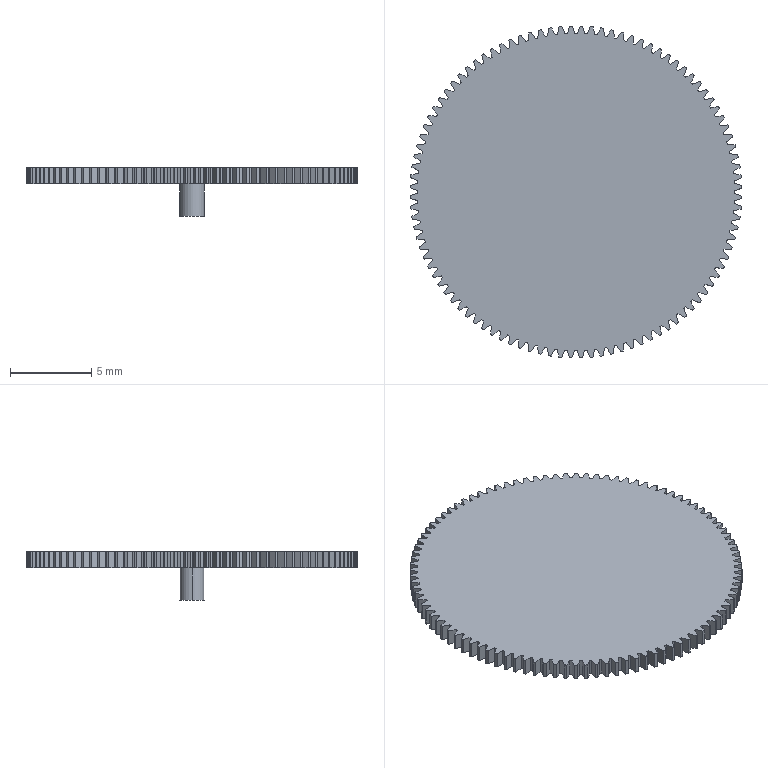Part | SolidWorks | features ICE 2, CirPattern 1, Extrusion 1 | 1 solid | 406 faces | box 20.395 x 20.395 x 3 mm | volume 316.823 mm3 | cylinder 203 | spline 200 | plane 3 | commonest cylinder face diameters 19.5 x101 20.4 x100 1.5 x2